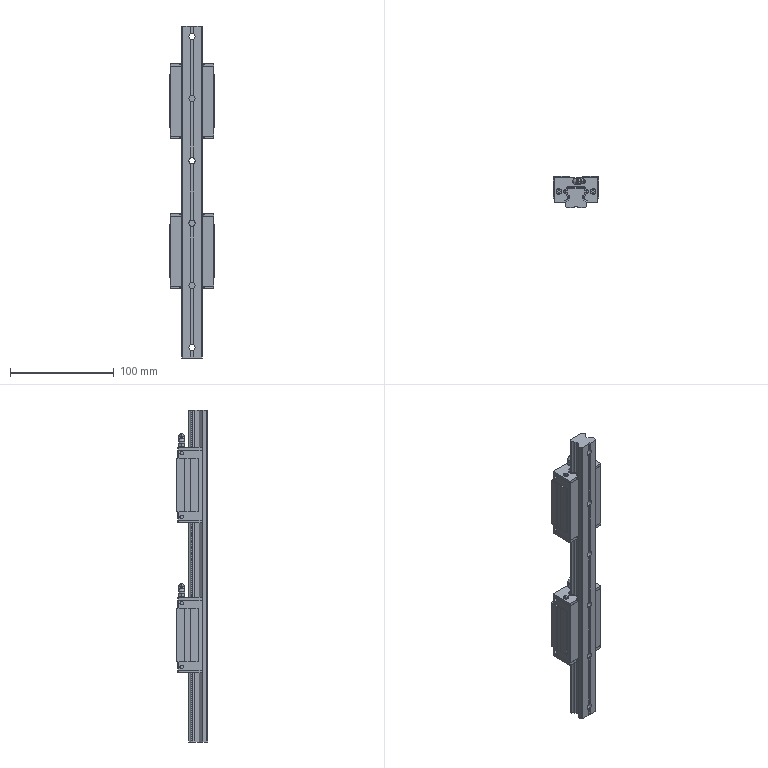Part | SolidWorks | 3 solids | 763 faces | box 44 x 29.99 x 320 mm | volume 212092 mm3 | plane 514 | cylinder 141 | cone 102 | spline 6 | commonest cylinder face diameters 5 x32 6 x20 3.3 x16 5.4 x16 4.455 x12 9.5 x12